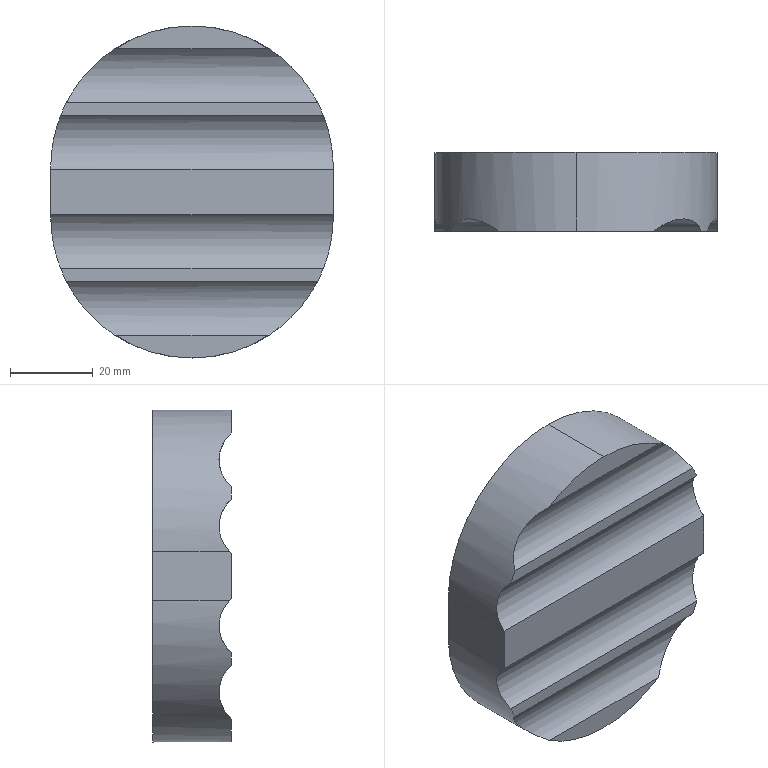Part | SolidWorks | features MirrorStock 1 | 1 solid | 22 faces | box 68 x 19 x 80 mm | volume 59636 mm3 | cylinder 11 | plane 9 | cone 2 | commonest cylinder face diameters 17 x4 68 x3 8.5 x2 62 x2
STEP:
#1=CARTESIAN_POINT('',(0.,7.,-4.25));
#2=VERTEX_POINT('',#1);
#3=CARTESIAN_POINT('',(0.,7.,4.25));
#4=VERTEX_POINT('',#3);
#5=CARTESIAN_POINT('',(0.,7.,0.));
#6=DIRECTION('',(0.,-1.,0.));
#7=DIRECTION('',(0.,0.,-1.));
#8=AXIS2_PLACEMENT_3D('',#5,#6,#7);
#9=CIRCLE('',#8,4.25);
#10=EDGE_CURVE('',#2,#4,#9,.T.);
#11=ORIENTED_EDGE('',*,*,#10,.T.);
#12=CARTESIAN_POINT('',(0.,13.,4.25));
#13=VERTEX_POINT('',#12);
#14=CARTESIAN_POINT('',(0.,13.,4.25));
#15=DIRECTION('',(0.,1.,0.));
#16=VECTOR('',#15,1000.);
#17=LINE('',#14,#16);
#18=EDGE_CURVE('',#4,#13,#17,.T.);
#19=ORIENTED_EDGE('',*,*,#18,.T.);
#20=CARTESIAN_POINT('',(0.,13.,-4.25));
#21=VERTEX_POINT('',#20);
#22=CARTESIAN_POINT('',(0.,13.,0.));
#23=DIRECTION('',(0.,-1.,0.));
#24=DIRECTION('',(0.,0.,-1.));
#25=AXIS2_PLACEMENT_3D('',#22,#23,#24);
#26=CIRCLE('',#25,4.25);
#27=EDGE_CURVE('',#21,#13,#26,.T.);
#28=ORIENTED_EDGE('',*,*,#27,.F.);
#29=CARTESIAN_POINT('',(0.,13.,-4.25));
#30=DIRECTION('',(0.,1.,0.));
#31=VECTOR('',#30,1000.);
#32=LINE('',#29,#31);
#33=EDGE_CURVE('',#2,#21,#32,.T.);
#34=ORIENTED_EDGE('',*,*,#33,.F.);
#35=EDGE_LOOP('',(#11,#19,#28,#34));
#36=FACE_OUTER_BOUND('',#35,.T.);
#37=CARTESIAN_POINT('',(0.,13.,0.));
#38=DIRECTION('',(0.,1.,0.));
#39=DIRECTION('',(0.,0.,-1.));
#40=AXIS2_PLACEMENT_3D('',#37,#38,#39);
#41=CYLINDRICAL_SURFACE('',#40,4.25);
#42=ADVANCED_FACE('',(#36),#41,.F.);
#43=CARTESIAN_POINT('',(0.,4.446,0.));
#44=VERTEX_POINT('',#43);
#45=CARTESIAN_POINT('',(0.,7.,-4.25));
#46=DIRECTION('',(0.,0.515,-0.8572));
#47=VECTOR('',#46,1000.);
#48=LINE('',#45,#47);
#49=EDGE_CURVE('',#44,#2,#48,.T.);
#50=ORIENTED_EDGE('',*,*,#49,.F.);
#51=CARTESIAN_POINT('',(0.,7.,4.25));
#52=DIRECTION('',(0.,0.515,0.8572));
#53=VECTOR('',#52,1000.);
#54=LINE('',#51,#53);
#55=EDGE_CURVE('',#44,#4,#54,.T.);
#56=ORIENTED_EDGE('',*,*,#55,.T.);
#57=ORIENTED_EDGE('',*,*,#10,.F.);
#58=EDGE_LOOP('',(#50,#56,#57));
#59=FACE_OUTER_BOUND('',#58,.T.);
#60=CARTESIAN_POINT('',(0.,7.,0.));
#61=DIRECTION('',(0.,1.,0.));
#62=DIRECTION('',(0.,0.,-1.));
#63=AXIS2_PLACEMENT_3D('',#60,#61,#62);
#64=CONICAL_SURFACE('',#63,4.25,1.03);
#65=ADVANCED_FACE('',(#59),#64,.F.);
#66=CARTESIAN_POINT('',(0.,13.,-31.));
#67=VERTEX_POINT('',#66);
#68=CARTESIAN_POINT('',(0.,13.,31.));
#69=VERTEX_POINT('',#68);
#70=CARTESIAN_POINT('',(0.,13.,0.));
#71=DIRECTION('',(0.,-1.,0.));
#72=DIRECTION('',(0.,0.,-1.));
#73=AXIS2_PLACEMENT_3D('',#70,#71,#72);
#74=CIRCLE('',#73,31.);
#75=EDGE_CURVE('',#67,#69,#74,.T.);
#76=ORIENTED_EDGE('',*,*,#75,.T.);
#77=CARTESIAN_POINT('',(0.,19.,31.));
#78=VERTEX_POINT('',#77);
#79=CARTESIAN_POINT('',(0.,13.,31.));
#80=DIRECTION('',(0.,1.,0.));
#81=VECTOR('',#80,1000.);
#82=LINE('',#79,#81);
#83=EDGE_CURVE('',#69,#78,#82,.T.);
#84=ORIENTED_EDGE('',*,*,#83,.T.);
#85=CARTESIAN_POINT('',(0.,19.,-31.));
#86=VERTEX_POINT('',#85);
#87=CARTESIAN_POINT('',(0.,19.,0.));
#88=DIRECTION('',(0.,-1.,0.));
#89=DIRECTION('',(0.,0.,-1.));
#90=AXIS2_PLACEMENT_3D('',#87,#88,#89);
#91=CIRCLE('',#90,31.);
#92=EDGE_CURVE('',#86,#78,#91,.T.);
#93=ORIENTED_EDGE('',*,*,#92,.F.);
#94=CARTESIAN_POINT('',(0.,13.,-31.));
#95=DIRECTION('',(0.,1.,0.));
#96=VECTOR('',#95,1000.);
#97=LINE('',#94,#96);
#98=EDGE_CURVE('',#67,#86,#97,.T.);
#99=ORIENTED_EDGE('',*,*,#98,.F.);
#100=EDGE_LOOP('',(#76,#84,#93,#99));
#101=FACE_OUTER_BOUND('',#100,.T.);
#102=CARTESIAN_POINT('',(0.,13.,0.));
#103=DIRECTION('',(0.,1.,0.));
#104=DIRECTION('',(0.,0.,-1.));
#105=AXIS2_PLACEMENT_3D('',#102,#103,#104);
#106=CYLINDRICAL_SURFACE('',#105,31.);
#107=ADVANCED_FACE('',(#101),#106,.F.);
#108=CARTESIAN_POINT('',(34.,19.,6.));
#109=VERTEX_POINT('',#108);
#110=CARTESIAN_POINT('',(0.,19.,40.));
#111=VERTEX_POINT('',#110);
#112=CARTESIAN_POINT('',(0.,19.,6.));
#113=DIRECTION('',(0.,-1.,0.));
#114=DIRECTION('',(0.,0.,-1.));
#115=AXIS2_PLACEMENT_3D('',#112,#113,#114);
#116=CIRCLE('',#115,34.);
#117=EDGE_CURVE('',#109,#111,#116,.T.);
#118=ORIENTED_EDGE('',*,*,#117,.T.);
#119=CARTESIAN_POINT('',(0.,0.,40.));
#120=VERTEX_POINT('',#119);
#121=CARTESIAN_POINT('',(0.,19.,40.));
#122=DIRECTION('',(0.,-1.,0.));
#123=VECTOR('',#122,1000.);
#124=LINE('',#121,#123);
#125=EDGE_CURVE('',#111,#120,#124,.T.);
#126=ORIENTED_EDGE('',*,*,#125,.T.);
#127=CARTESIAN_POINT('',(18.57,0.,34.481));
#128=VERTEX_POINT('',#127);
#129=CARTESIAN_POINT('',(0.,0.,6.));
#130=DIRECTION('',(0.,-1.,0.));
#131=DIRECTION('',(0.,0.,-1.));
#132=AXIS2_PLACEMENT_3D('',#129,#130,#131);
#133=CIRCLE('',#132,34.);
#134=EDGE_CURVE('',#128,#120,#133,.T.);
#135=ORIENTED_EDGE('',*,*,#134,.F.);
#136=CARTESIAN_POINT('',(30.251,0.,21.519));
#137=VERTEX_POINT('',#136);
#138=CARTESIAN_POINT('',(18.57,0.,34.481));
#139=CARTESIAN_POINT('',(19.132,0.4318,34.114));
#140=CARTESIAN_POINT('',(19.701,0.8113,33.719));
#141=CARTESIAN_POINT('',(20.842,1.486,32.872));
#142=CARTESIAN_POINT('',(21.414,1.781,32.419));
#143=CARTESIAN_POINT('',(22.557,2.287,31.451));
#144=CARTESIAN_POINT('',(23.13,2.498,30.932));
#145=CARTESIAN_POINT('',(24.241,2.815,29.853));
#146=CARTESIAN_POINT('',(24.783,2.922,29.29));
#147=CARTESIAN_POINT('',(25.572,2.995,28.41));
#148=CARTESIAN_POINT('',(25.832,3.005,28.111));
#149=CARTESIAN_POINT('',(26.343,2.991,27.499));
#150=CARTESIAN_POINT('',(26.593,2.967,27.189));
#151=CARTESIAN_POINT('',(27.319,2.843,26.256));
#152=CARTESIAN_POINT('',(27.773,2.69,25.628));
#153=CARTESIAN_POINT('',(28.41,2.333,24.682));
#154=CARTESIAN_POINT('',(28.615,2.192,24.366));
#155=CARTESIAN_POINT('',(29.,1.871,23.752));
#156=CARTESIAN_POINT('',(29.182,1.689,23.451));
#157=CARTESIAN_POINT('',(29.524,1.283,22.865));
#158=CARTESIAN_POINT('',(29.686,1.057,22.579));
#159=CARTESIAN_POINT('',(29.987,0.5594,22.027));
#160=CARTESIAN_POINT('',(30.125,0.2903,21.766));
#161=CARTESIAN_POINT('',(30.251,0.,21.519));
#162=B_SPLINE_CURVE_WITH_KNOTS('',3,(#138,#139,#140,#141,#142,#143,#144,#145,#146,#147,#148,#149,#150,#151,#152,#153,#154,#155,#156,#157,#158,#159,#160,#161),.UNSPECIFIED.,.F.,.F.,(4,2,2,2,2,2,2,2,2,2,2,4),(0.,0.002359,0.004718,0.007077,0.009436,0.01062,0.0118,0.01415,0.01533,0.01651,0.01769,0.01887),.UNSPECIFIED.);
#163=EDGE_CURVE('',#128,#137,#162,.T.);
#164=ORIENTED_EDGE('',*,*,#163,.T.);
#165=CARTESIAN_POINT('',(31.626,0.,18.481));
#166=VERTEX_POINT('',#165);
#167=CARTESIAN_POINT('',(0.,0.,6.));
#168=DIRECTION('',(0.,-1.,0.));
#169=DIRECTION('',(0.,0.,-1.));
#170=AXIS2_PLACEMENT_3D('',#167,#168,#169);
#171=CIRCLE('',#170,34.);
#172=EDGE_CURVE('',#166,#137,#171,.T.);
#173=ORIENTED_EDGE('',*,*,#172,.F.);
#174=CARTESIAN_POINT('',(34.,0.5208,6.));
#175=VERTEX_POINT('',#174);
#176=CARTESIAN_POINT('',(31.626,0.,18.481));
#177=CARTESIAN_POINT('',(31.775,0.4439,18.104));
#178=CARTESIAN_POINT('',(31.931,0.8401,17.69));
#179=CARTESIAN_POINT('',(32.167,1.368,17.016));
#180=CARTESIAN_POINT('',(32.246,1.533,16.782));
#181=CARTESIAN_POINT('',(32.405,1.841,16.295));
#182=CARTESIAN_POINT('',(32.484,1.983,16.042));
#183=CARTESIAN_POINT('',(32.717,2.367,15.269));
#184=CARTESIAN_POINT('',(32.865,2.57,14.732));
#185=CARTESIAN_POINT('',(33.072,2.791,13.894));
#186=CARTESIAN_POINT('',(33.139,2.852,13.608));
#187=CARTESIAN_POINT('',(33.267,2.943,13.029));
#188=CARTESIAN_POINT('',(33.327,2.973,12.739));
#189=CARTESIAN_POINT('',(33.495,3.019,11.868));
#190=CARTESIAN_POINT('',(33.592,2.991,11.284));
#191=CARTESIAN_POINT('',(33.715,2.854,10.405));
#192=CARTESIAN_POINT('',(33.752,2.793,10.113));
#193=CARTESIAN_POINT('',(33.816,2.642,9.541));
#194=CARTESIAN_POINT('',(33.844,2.552,9.26));
#195=CARTESIAN_POINT('',(33.893,2.342,8.708));
#196=CARTESIAN_POINT('',(33.914,2.223,8.437));
#197=CARTESIAN_POINT('',(33.948,1.954,7.905));
#198=CARTESIAN_POINT('',(33.961,1.805,7.643));
#199=CARTESIAN_POINT('',(33.992,1.319,6.89));
#200=CARTESIAN_POINT('',(34.,0.9452,6.426));
#201=CARTESIAN_POINT('',(34.,0.5208,6.));
#202=B_SPLINE_CURVE_WITH_KNOTS('',3,(#176,#177,#178,#179,#180,#181,#182,#183,#184,#185,#186,#187,#188,#189,#190,#191,#192,#193,#194,#195,#196,#197,#198,#199,#200,#201),.UNSPECIFIED.,.F.,.F.,(4,2,2,2,2,2,2,2,2,2,2,2,4),(0.,0.001777,0.002665,0.003554,0.005331,0.006219,0.007107,0.008884,0.009773,0.01066,0.01155,0.01244,0.01421),.UNSPECIFIED.);
#203=EDGE_CURVE('',#166,#175,#202,.T.);
#204=ORIENTED_EDGE('',*,*,#203,.T.);
#205=CARTESIAN_POINT('',(34.,19.,6.));
#206=DIRECTION('',(0.,-1.,0.));
#207=VECTOR('',#206,1000.);
#208=LINE('',#205,#207);
#209=EDGE_CURVE('',#109,#175,#208,.T.);
#210=ORIENTED_EDGE('',*,*,#209,.F.);
#211=EDGE_LOOP('',(#118,#126,#135,#164,#173,#204,#210));
#212=FACE_OUTER_BOUND('',#211,.T.);
#213=CARTESIAN_POINT('',(0.,19.,6.));
#214=DIRECTION('',(0.,-1.,0.));
#215=DIRECTION('',(0.,0.,1.));
#216=AXIS2_PLACEMENT_3D('',#213,#214,#215);
#217=CYLINDRICAL_SURFACE('',#216,34.);
#218=ADVANCED_FACE('',(#212),#217,.T.);
#219=ORIENTED_EDGE('',*,*,#125,.F.);
#220=CARTESIAN_POINT('',(-34.,19.,6.));
#221=VERTEX_POINT('',#220);
#222=CARTESIAN_POINT('',(0.,19.,6.));
#223=DIRECTION('',(0.,-1.,0.));
#224=DIRECTION('',(0.,0.,-1.));
#225=AXIS2_PLACEMENT_3D('',#222,#223,#224);
#226=CIRCLE('',#225,34.);
#227=EDGE_CURVE('',#111,#221,#226,.T.);
#228=ORIENTED_EDGE('',*,*,#227,.T.);
#229=CARTESIAN_POINT('',(-34.,0.5208,6.));
#230=VERTEX_POINT('',#229);
#231=CARTESIAN_POINT('',(-34.,19.,6.));
#232=DIRECTION('',(0.,-1.,0.));
#233=VECTOR('',#232,1000.);
#234=LINE('',#231,#233);
#235=EDGE_CURVE('',#221,#230,#234,.T.);
#236=ORIENTED_EDGE('',*,*,#235,.T.);
#237=CARTESIAN_POINT('',(-31.626,0.,18.481));
#238=VERTEX_POINT('',#237);
#239=CARTESIAN_POINT('',(-34.,0.5208,6.));
#240=CARTESIAN_POINT('',(-34.,0.9451,6.426));
#241=CARTESIAN_POINT('',(-33.992,1.317,6.888));
#242=CARTESIAN_POINT('',(-33.962,1.8,7.635));
#243=CARTESIAN_POINT('',(-33.948,1.948,7.893));
#244=CARTESIAN_POINT('',(-33.914,2.218,8.427));
#245=CARTESIAN_POINT('',(-33.894,2.339,8.701));
#246=CARTESIAN_POINT('',(-33.821,2.655,9.532));
#247=CARTESIAN_POINT('',(-33.757,2.806,10.101));
#248=CARTESIAN_POINT('',(-33.635,2.944,10.979));
#249=CARTESIAN_POINT('',(-33.59,2.974,11.276));
#250=CARTESIAN_POINT('',(-33.492,3.004,11.862));
#251=CARTESIAN_POINT('',(-33.44,3.004,12.154));
#252=CARTESIAN_POINT('',(-33.327,2.973,12.736));
#253=CARTESIAN_POINT('',(-33.268,2.943,13.025));
#254=CARTESIAN_POINT('',(-33.141,2.853,13.601));
#255=CARTESIAN_POINT('',(-33.073,2.792,13.889));
#256=CARTESIAN_POINT('',(-32.865,2.57,14.73));
#257=CARTESIAN_POINT('',(-32.717,2.368,15.268));
#258=CARTESIAN_POINT('',(-32.485,1.984,16.04));
#259=CARTESIAN_POINT('',(-32.405,1.842,16.293));
#260=CARTESIAN_POINT('',(-32.247,1.534,16.781));
#261=CARTESIAN_POINT('',(-32.167,1.369,17.015));
#262=CARTESIAN_POINT('',(-31.931,0.8402,17.69));
#263=CARTESIAN_POINT('',(-31.775,0.4438,18.104));
#264=CARTESIAN_POINT('',(-31.626,0.,18.481));
#265=B_SPLINE_CURVE_WITH_KNOTS('',3,(#239,#240,#241,#242,#243,#244,#245,#246,#247,#248,#249,#250,#251,#252,#253,#254,#255,#256,#257,#258,#259,#260,#261,#262,#263,#264),.UNSPECIFIED.,.F.,.F.,(4,2,2,2,2,2,2,2,2,2,2,2,4),(0.,0.001778,0.002667,0.003556,0.005334,0.006222,0.007111,0.008,0.008889,0.01067,0.01156,0.01244,0.01422),.UNSPECIFIED.);
#266=EDGE_CURVE('',#230,#238,#265,.T.);
#267=ORIENTED_EDGE('',*,*,#266,.T.);
#268=CARTESIAN_POINT('',(-30.251,0.,21.519));
#269=VERTEX_POINT('',#268);
#270=CARTESIAN_POINT('',(0.,0.,6.));
#271=DIRECTION('',(0.,-1.,0.));
#272=DIRECTION('',(0.,0.,-1.));
#273=AXIS2_PLACEMENT_3D('',#270,#271,#272);
#274=CIRCLE('',#273,34.);
#275=EDGE_CURVE('',#269,#238,#274,.T.);
#276=ORIENTED_EDGE('',*,*,#275,.F.);
#277=CARTESIAN_POINT('',(-18.57,0.,34.481));
#278=VERTEX_POINT('',#277);
#279=CARTESIAN_POINT('',(-30.251,0.,21.519));
#280=CARTESIAN_POINT('',(-29.999,0.5804,22.012));
#281=CARTESIAN_POINT('',(-29.703,1.069,22.558));
#282=CARTESIAN_POINT('',(-29.189,1.681,23.438));
#283=CARTESIAN_POINT('',(-29.005,1.866,23.744));
#284=CARTESIAN_POINT('',(-28.619,2.189,24.361));
#285=CARTESIAN_POINT('',(-28.417,2.328,24.672));
#286=CARTESIAN_POINT('',(-27.995,2.566,25.298));
#287=CARTESIAN_POINT('',(-27.775,2.665,25.614));
#288=CARTESIAN_POINT('',(-27.317,2.824,26.247));
#289=CARTESIAN_POINT('',(-27.08,2.884,26.563));
#290=CARTESIAN_POINT('',(-26.355,3.008,27.495));
#291=CARTESIAN_POINT('',(-25.85,3.02,28.1));
#292=CARTESIAN_POINT('',(-25.059,2.948,28.982));
#293=CARTESIAN_POINT('',(-24.789,2.909,29.273));
#294=CARTESIAN_POINT('',(-24.243,2.803,29.842));
#295=CARTESIAN_POINT('',(-23.967,2.736,30.119));
#296=CARTESIAN_POINT('',(-23.136,2.5,30.927));
#297=CARTESIAN_POINT('',(-22.573,2.293,31.436));
#298=CARTESIAN_POINT('',(-21.72,1.917,32.161));
#299=CARTESIAN_POINT('',(-21.433,1.78,32.396));
#300=CARTESIAN_POINT('',(-20.858,1.484,32.853));
#301=CARTESIAN_POINT('',(-20.568,1.324,33.075));
#302=CARTESIAN_POINT('',(-19.703,0.8129,33.718));
#303=CARTESIAN_POINT('',(-19.131,0.4312,34.115));
#304=CARTESIAN_POINT('',(-18.57,0.,34.481));
#305=B_SPLINE_CURVE_WITH_KNOTS('',3,(#279,#280,#281,#282,#283,#284,#285,#286,#287,#288,#289,#290,#291,#292,#293,#294,#295,#296,#297,#298,#299,#300,#301,#302,#303,#304),.UNSPECIFIED.,.F.,.F.,(4,2,2,2,2,2,2,2,2,2,2,2,4),(0.,0.002368,0.003552,0.004736,0.005921,0.007105,0.009473,0.01066,0.01184,0.01421,0.01539,0.01658,0.01895),.UNSPECIFIED.);
#306=EDGE_CURVE('',#269,#278,#305,.T.);
#307=ORIENTED_EDGE('',*,*,#306,.T.);
#308=CARTESIAN_POINT('',(0.,0.,6.));
#309=DIRECTION('',(0.,-1.,0.));
#310=DIRECTION('',(0.,0.,-1.));
#311=AXIS2_PLACEMENT_3D('',#308,#309,#310);
#312=CIRCLE('',#311,34.);
#313=EDGE_CURVE('',#120,#278,#312,.T.);
#314=ORIENTED_EDGE('',*,*,#313,.F.);
#315=EDGE_LOOP('',(#219,#228,#236,#267,#276,#307,#314));
#316=FACE_OUTER_BOUND('',#315,.T.);
#317=CARTESIAN_POINT('',(0.,19.,6.));
#318=DIRECTION('',(0.,-1.,0.));
#319=DIRECTION('',(0.,0.,1.));
#320=AXIS2_PLACEMENT_3D('',#317,#318,#319);
#321=CYLINDRICAL_SURFACE('',#320,34.);
#322=ADVANCED_FACE('',(#316),#321,.T.);
#323=CARTESIAN_POINT('',(34.,0.,5.519));
#324=VERTEX_POINT('',#323);
#325=CARTESIAN_POINT('',(-34.,0.,5.519));
#326=VERTEX_POINT('',#325);
#327=CARTESIAN_POINT('',(-34.,0.,5.519));
#328=DIRECTION('',(-1.,0.,0.));
#329=VECTOR('',#328,1000.);
#330=LINE('',#327,#329);
#331=EDGE_CURVE('',#324,#326,#330,.T.);
#332=ORIENTED_EDGE('',*,*,#331,.T.);
#333=CARTESIAN_POINT('',(-34.,0.,-5.519));
#334=VERTEX_POINT('',#333);
#335=CARTESIAN_POINT('',(-34.,0.,-6.));
#336=DIRECTION('',(0.,0.,-1.));
#337=VECTOR('',#336,1000.);
#338=LINE('',#335,#337);
#339=EDGE_CURVE('',#326,#334,#338,.T.);
#340=ORIENTED_EDGE('',*,*,#339,.T.);
#341=CARTESIAN_POINT('',(34.,0.,-5.519));
#342=VERTEX_POINT('',#341);
#343=CARTESIAN_POINT('',(-34.,0.,-5.519));
#344=DIRECTION('',(-1.,0.,0.));
#345=VECTOR('',#344,1000.);
#346=LINE('',#343,#345);
#347=EDGE_CURVE('',#342,#334,#346,.T.);
#348=ORIENTED_EDGE('',*,*,#347,.F.);
#349=CARTESIAN_POINT('',(34.,0.,-6.));
#350=DIRECTION('',(0.,0.,1.));
#351=VECTOR('',#350,1000.);
#352=LINE('',#349,#351);
#353=EDGE_CURVE('',#342,#324,#352,.T.);
#354=ORIENTED_EDGE('',*,*,#353,.T.);
#355=EDGE_LOOP('',(#332,#340,#348,#354));
#356=FACE_OUTER_BOUND('',#355,.T.);
#357=CARTESIAN_POINT('',(0.,0.,6.));
#358=DIRECTION('',(0.,1.,0.));
#359=DIRECTION('',(0.,0.,-1.));
#360=AXIS2_PLACEMENT_3D('',#357,#358,#359);
#361=PLANE('',#360);
#362=ADVANCED_FACE('',(#356),#361,.F.);
#363=CARTESIAN_POINT('',(-34.,0.,18.481));
#364=DIRECTION('',(1.,0.,0.));
#365=VECTOR('',#364,1000.);
#366=LINE('',#363,#365);
#367=EDGE_CURVE('',#238,#166,#366,.T.);
#368=ORIENTED_EDGE('',*,*,#367,.T.);
#369=ORIENTED_EDGE('',*,*,#172,.T.);
#370=CARTESIAN_POINT('',(-34.,0.,21.519));
#371=DIRECTION('',(-1.,0.,0.));
#372=VECTOR('',#371,1000.);
#373=LINE('',#370,#372);
#374=EDGE_CURVE('',#137,#269,#373,.T.);
#375=ORIENTED_EDGE('',*,*,#374,.T.);
#376=ORIENTED_EDGE('',*,*,#275,.T.);
#377=EDGE_LOOP('',(#368,#369,#375,#376));
#378=FACE_OUTER_BOUND('',#377,.T.);
#379=CARTESIAN_POINT('',(0.,0.,6.));
#380=DIRECTION('',(0.,1.,0.));
#381=DIRECTION('',(0.,0.,-1.));
#382=AXIS2_PLACEMENT_3D('',#379,#380,#381);
#383=PLANE('',#382);
#384=ADVANCED_FACE('',(#378),#383,.F.);
#385=CARTESIAN_POINT('',(-31.626,0.,-18.481));
#386=VERTEX_POINT('',#385);
#387=CARTESIAN_POINT('',(-30.251,0.,-21.519));
#388=VERTEX_POINT('',#387);
#389=CARTESIAN_POINT('',(0.,0.,-6.));
#390=DIRECTION('',(0.,-1.,0.));
#391=DIRECTION('',(0.,0.,1.));
#392=AXIS2_PLACEMENT_3D('',#389,#390,#391);
#393=CIRCLE('',#392,34.);
#394=EDGE_CURVE('',#386,#388,#393,.T.);
#395=ORIENTED_EDGE('',*,*,#394,.T.);
#396=CARTESIAN_POINT('',(30.251,0.,-21.519));
#397=VERTEX_POINT('',#396);
#398=CARTESIAN_POINT('',(-34.,0.,-21.519));
#399=DIRECTION('',(-1.,0.,0.));
#400=VECTOR('',#399,1000.);
#401=LINE('',#398,#400);
#402=EDGE_CURVE('',#397,#388,#401,.T.);
#403=ORIENTED_EDGE('',*,*,#402,.F.);
#404=CARTESIAN_POINT('',(31.626,0.,-18.481));
#405=VERTEX_POINT('',#404);
#406=CARTESIAN_POINT('',(0.,0.,-6.));
#407=DIRECTION('',(0.,-1.,0.));
#408=DIRECTION('',(0.,0.,1.));
#409=AXIS2_PLACEMENT_3D('',#406,#407,#408);
#410=CIRCLE('',#409,34.);
#411=EDGE_CURVE('',#397,#405,#410,.T.);
#412=ORIENTED_EDGE('',*,*,#411,.T.);
#413=CARTESIAN_POINT('',(-34.,0.,-18.481));
#414=DIRECTION('',(1.,0.,0.));
#415=VECTOR('',#414,1000.);
#416=LINE('',#413,#415);
#417=EDGE_CURVE('',#386,#405,#416,.T.);
#418=ORIENTED_EDGE('',*,*,#417,.F.);
#419=EDGE_LOOP('',(#395,#403,#412,#418));
#420=FACE_OUTER_BOUND('',#419,.T.);
#421=CARTESIAN_POINT('',(0.,0.,6.));
#422=DIRECTION('',(0.,1.,0.));
#423=DIRECTION('',(0.,0.,-1.));
#424=AXIS2_PLACEMENT_3D('',#421,#422,#423);
#425=PLANE('',#424);
#426=ADVANCED_FACE('',(#420),#425,.F.);
#427=CARTESIAN_POINT('',(-34.,-5.5,12.));
#428=DIRECTION('',(1.,0.,0.));
#429=DIRECTION('',(0.,0.,1.));
#430=AXIS2_PLACEMENT_3D('',#427,#428,#429);
#431=CIRCLE('',#430,8.5);
#432=EDGE_CURVE('',#326,#230,#431,.T.);
#433=ORIENTED_EDGE('',*,*,#432,.T.);
#434=ORIENTED_EDGE('',*,*,#235,.F.);
#435=CARTESIAN_POINT('',(-34.,19.,-6.));
#436=VERTEX_POINT('',#435);
#437=CARTESIAN_POINT('',(-34.,19.,-6.));
#438=DIRECTION('',(0.,0.,-1.));
#439=VECTOR('',#438,1000.);
#440=LINE('',#437,#439);
#441=EDGE_CURVE('',#221,#436,#440,.T.);
#442=ORIENTED_EDGE('',*,*,#441,.T.);
#443=CARTESIAN_POINT('',(-34.,0.5208,-6.));
#444=VERTEX_POINT('',#443);
#445=CARTESIAN_POINT('',(-34.,19.,-6.));
#446=DIRECTION('',(0.,-1.,0.));
#447=VECTOR('',#446,1000.);
#448=LINE('',#445,#447);
#449=EDGE_CURVE('',#436,#444,#448,.T.);
#450=ORIENTED_EDGE('',*,*,#449,.T.);
#451=CARTESIAN_POINT('',(-34.,-5.5,-12.));
#452=DIRECTION('',(-1.,0.,0.));
#453=DIRECTION('',(0.,0.,1.));
#454=AXIS2_PLACEMENT_3D('',#451,#452,#453);
#455=CIRCLE('',#454,8.5);
#456=EDGE_CURVE('',#334,#444,#455,.T.);
#457=ORIENTED_EDGE('',*,*,#456,.F.);
#458=ORIENTED_EDGE('',*,*,#339,.F.);
#459=EDGE_LOOP('',(#433,#434,#442,#450,#457,#458));
#460=FACE_OUTER_BOUND('',#459,.T.);
#461=CARTESIAN_POINT('',(-34.,19.,-6.));
#462=DIRECTION('',(1.,0.,0.));
#463=DIRECTION('',(0.,0.,1.));
#464=AXIS2_PLACEMENT_3D('',#461,#462,#463);
#465=PLANE('',#464);
#466=ADVANCED_FACE('',(#460),#465,.F.);
#467=CARTESIAN_POINT('',(34.,-5.5,12.));
#468=DIRECTION('',(-1.,0.,0.));
#469=DIRECTION('',(0.,0.,-1.));
#470=AXIS2_PLACEMENT_3D('',#467,#468,#469);
#471=CIRCLE('',#470,8.5);
#472=EDGE_CURVE('',#175,#324,#471,.T.);
#473=ORIENTED_EDGE('',*,*,#472,.T.);
#474=ORIENTED_EDGE('',*,*,#353,.F.);
#475=CARTESIAN_POINT('',(34.,0.5208,-6.));
#476=VERTEX_POINT('',#475);
#477=CARTESIAN_POINT('',(34.,-5.5,-12.));
#478=DIRECTION('',(1.,0.,0.));
#479=DIRECTION('',(0.,0.,-1.));
#480=AXIS2_PLACEMENT_3D('',#477,#478,#479);
#481=CIRCLE('',#480,8.5);
#482=EDGE_CURVE('',#476,#342,#481,.T.);
#483=ORIENTED_EDGE('',*,*,#482,.F.);
#484=CARTESIAN_POINT('',(34.,19.,-6.));
#485=VERTEX_POINT('',#484);
#486=CARTESIAN_POINT('',(34.,19.,-6.));
#487=DIRECTION('',(0.,-1.,0.));
#488=VECTOR('',#487,1000.);
#489=LINE('',#486,#488);
#490=EDGE_CURVE('',#485,#476,#489,.T.);
#491=ORIENTED_EDGE('',*,*,#490,.F.);
#492=CARTESIAN_POINT('',(34.,19.,-6.));
#493=DIRECTION('',(0.,0.,1.));
#494=VECTOR('',#493,1000.);
#495=LINE('',#492,#494);
#496=EDGE_CURVE('',#485,#109,#495,.T.);
#497=ORIENTED_EDGE('',*,*,#496,.T.);
#498=ORIENTED_EDGE('',*,*,#209,.T.);
#499=EDGE_LOOP('',(#473,#474,#483,#491,#497,#498));
#500=FACE_OUTER_BOUND('',#499,.T.);
#501=CARTESIAN_POINT('',(34.,19.,-6.));
#502=DIRECTION('',(-1.,0.,0.));
#503=DIRECTION('',(0.,0.,-1.));
#504=AXIS2_PLACEMENT_3D('',#501,#502,#503);
#505=PLANE('',#504);
#506=ADVANCED_FACE('',(#500),#505,.F.);
#507=CARTESIAN_POINT('',(-34.,0.,34.481));
#508=DIRECTION('',(1.,0.,0.));
#509=VECTOR('',#508,1000.);
#510=LINE('',#507,#509);
#511=EDGE_CURVE('',#278,#128,#510,.T.);
#512=ORIENTED_EDGE('',*,*,#511,.T.);
#513=ORIENTED_EDGE('',*,*,#134,.T.);
#514=ORIENTED_EDGE('',*,*,#313,.T.);
#515=EDGE_LOOP('',(#512,#513,#514));
#516=FACE_OUTER_BOUND('',#515,.T.);
#517=CARTESIAN_POINT('',(0.,0.,6.));
#518=DIRECTION('',(0.,1.,0.));
#519=DIRECTION('',(0.,0.,-1.));
#520=AXIS2_PLACEMENT_3D('',#517,#518,#519);
#521=PLANE('',#520);
#522=ADVANCED_FACE('',(#516),#521,.F.);
#523=CARTESIAN_POINT('',(-18.57,0.,-34.481));
#524=VERTEX_POINT('',#523);
#525=CARTESIAN_POINT('',(18.57,0.,-34.481));
#526=VERTEX_POINT('',#525);
#527=CARTESIAN_POINT('',(0.,0.,-6.));
#528=DIRECTION('',(0.,-1.,0.));
#529=DIRECTION('',(0.,0.,1.));
#530=AXIS2_PLACEMENT_3D('',#527,#528,#529);
#531=CIRCLE('',#530,34.);
#532=EDGE_CURVE('',#524,#526,#531,.T.);
#533=ORIENTED_EDGE('',*,*,#532,.T.);
#534=CARTESIAN_POINT('',(-34.,0.,-34.481));
#535=DIRECTION('',(1.,0.,0.));
#536=VECTOR('',#535,1000.);
#537=LINE('',#534,#536);
#538=EDGE_CURVE('',#524,#526,#537,.T.);
#539=ORIENTED_EDGE('',*,*,#538,.F.);
#540=EDGE_LOOP('',(#533,#539));
#541=FACE_OUTER_BOUND('',#540,.T.);
#542=CARTESIAN_POINT('',(0.,0.,6.));
#543=DIRECTION('',(0.,1.,0.));
#544=DIRECTION('',(0.,0.,-1.));
#545=AXIS2_PLACEMENT_3D('',#542,#543,#544);
#546=PLANE('',#545);
#547=ADVANCED_FACE('',(#541),#546,.F.);
#548=ORIENTED_EDGE('',*,*,#449,.F.);
#549=CARTESIAN_POINT('',(0.,19.,-6.));
#550=DIRECTION('',(0.,-1.,0.));
#551=DIRECTION('',(0.,0.,1.));
#552=AXIS2_PLACEMENT_3D('',#549,#550,#551);
#553=CIRCLE('',#552,34.);
#554=EDGE_CURVE('',#436,#485,#553,.T.);
#555=ORIENTED_EDGE('',*,*,#554,.T.);
#556=ORIENTED_EDGE('',*,*,#490,.T.);
#557=CARTESIAN_POINT('',(31.626,0.,-18.481));
#558=CARTESIAN_POINT('',(31.775,0.4439,-18.104));
#559=CARTESIAN_POINT('',(31.931,0.8401,-17.69));
#560=CARTESIAN_POINT('',(32.167,1.368,-17.016));
#561=CARTESIAN_POINT('',(32.246,1.533,-16.782));
#562=CARTESIAN_POINT('',(32.405,1.841,-16.295));
#563=CARTESIAN_POINT('',(32.484,1.983,-16.042));
#564=CARTESIAN_POINT('',(32.717,2.367,-15.269));
#565=CARTESIAN_POINT('',(32.865,2.57,-14.732));
#566=CARTESIAN_POINT('',(33.072,2.791,-13.894));
#567=CARTESIAN_POINT('',(33.139,2.852,-13.608));
#568=CARTESIAN_POINT('',(33.267,2.943,-13.029));
#569=CARTESIAN_POINT('',(33.327,2.973,-12.739));
#570=CARTESIAN_POINT('',(33.495,3.019,-11.868));
#571=CARTESIAN_POINT('',(33.592,2.991,-11.284));
#572=CARTESIAN_POINT('',(33.715,2.854,-10.405));
#573=CARTESIAN_POINT('',(33.752,2.793,-10.113));
#574=CARTESIAN_POINT('',(33.816,2.642,-9.541));
#575=CARTESIAN_POINT('',(33.844,2.552,-9.26));
#576=CARTESIAN_POINT('',(33.893,2.342,-8.708));
#577=CARTESIAN_POINT('',(33.914,2.223,-8.437));
#578=CARTESIAN_POINT('',(33.948,1.954,-7.905));
#579=CARTESIAN_POINT('',(33.961,1.805,-7.643));
#580=CARTESIAN_POINT('',(33.992,1.319,-6.89));
#581=CARTESIAN_POINT('',(34.,0.9452,-6.426));
#582=CARTESIAN_POINT('',(34.,0.5208,-6.));
#583=B_SPLINE_CURVE_WITH_KNOTS('',3,(#557,#558,#559,#560,#561,#562,#563,#564,#565,#566,#567,#568,#569,#570,#571,#572,#573,#574,#575,#576,#577,#578,#579,#580,#581,#582),.UNSPECIFIED.,.F.,.F.,(4,2,2,2,2,2,2,2,2,2,2,2,4),(0.,0.001777,0.002665,0.003554,0.005331,0.006219,0.007107,0.008884,0.009773,0.01066,0.01155,0.01244,0.01421),.UNSPECIFIED.);
#584=EDGE_CURVE('',#405,#476,#583,.T.);
#585=ORIENTED_EDGE('',*,*,#584,.F.);
#586=ORIENTED_EDGE('',*,*,#411,.F.);
#587=CARTESIAN_POINT('',(18.57,0.,-34.481));
#588=CARTESIAN_POINT('',(19.132,0.4318,-34.114));
#589=CARTESIAN_POINT('',(19.701,0.8113,-33.719));
#590=CARTESIAN_POINT('',(20.842,1.486,-32.872));
#591=CARTESIAN_POINT('',(21.414,1.781,-32.419));
#592=CARTESIAN_POINT('',(22.557,2.287,-31.451));
#593=CARTESIAN_POINT('',(23.13,2.498,-30.932));
#594=CARTESIAN_POINT('',(24.241,2.815,-29.853));
#595=CARTESIAN_POINT('',(24.783,2.922,-29.29));
#596=CARTESIAN_POINT('',(25.572,2.995,-28.41));
#597=CARTESIAN_POINT('',(25.832,3.005,-28.111));
#598=CARTESIAN_POINT('',(26.343,2.991,-27.499));
#599=CARTESIAN_POINT('',(26.593,2.967,-27.189));
#600=CARTESIAN_POINT('',(27.319,2.843,-26.256));
#601=CARTESIAN_POINT('',(27.773,2.69,-25.628));
#602=CARTESIAN_POINT('',(28.41,2.333,-24.682));
#603=CARTESIAN_POINT('',(28.615,2.192,-24.366));
#604=CARTESIAN_POINT('',(29.,1.871,-23.752));
#605=CARTESIAN_POINT('',(29.182,1.689,-23.451));
#606=CARTESIAN_POINT('',(29.524,1.283,-22.865));
#607=CARTESIAN_POINT('',(29.686,1.057,-22.579));
#608=CARTESIAN_POINT('',(29.987,0.5594,-22.027));
#609=CARTESIAN_POINT('',(30.125,0.2903,-21.766));
#610=CARTESIAN_POINT('',(30.251,0.,-21.519));
#611=B_SPLINE_CURVE_WITH_KNOTS('',3,(#587,#588,#589,#590,#591,#592,#593,#594,#595,#596,#597,#598,#599,#600,#601,#602,#603,#604,#605,#606,#607,#608,#609,#610),.UNSPECIFIED.,.F.,.F.,(4,2,2,2,2,2,2,2,2,2,2,4),(0.,0.002359,0.004718,0.007077,0.009436,0.01062,0.0118,0.01415,0.01533,0.01651,0.01769,0.01887),.UNSPECIFIED.);
#612=EDGE_CURVE('',#526,#397,#611,.T.);
#613=ORIENTED_EDGE('',*,*,#612,.F.);
#614=ORIENTED_EDGE('',*,*,#532,.F.);
#615=CARTESIAN_POINT('',(-30.251,0.,-21.519));
#616=CARTESIAN_POINT('',(-29.999,0.5804,-22.012));
#617=CARTESIAN_POINT('',(-29.703,1.069,-22.558));
#618=CARTESIAN_POINT('',(-29.189,1.681,-23.438));
#619=CARTESIAN_POINT('',(-29.005,1.866,-23.744));
#620=CARTESIAN_POINT('',(-28.619,2.189,-24.361));
#621=CARTESIAN_POINT('',(-28.417,2.328,-24.672));
#622=CARTESIAN_POINT('',(-27.995,2.566,-25.298));
#623=CARTESIAN_POINT('',(-27.775,2.665,-25.614));
#624=CARTESIAN_POINT('',(-27.317,2.824,-26.247));
#625=CARTESIAN_POINT('',(-27.08,2.884,-26.563));
#626=CARTESIAN_POINT('',(-26.355,3.008,-27.495));
#627=CARTESIAN_POINT('',(-25.85,3.02,-28.1));
#628=CARTESIAN_POINT('',(-25.059,2.948,-28.982));
#629=CARTESIAN_POINT('',(-24.789,2.909,-29.273));
#630=CARTESIAN_POINT('',(-24.243,2.803,-29.842));
#631=CARTESIAN_POINT('',(-23.967,2.736,-30.119));
#632=CARTESIAN_POINT('',(-23.136,2.5,-30.927));
#633=CARTESIAN_POINT('',(-22.573,2.293,-31.436));
#634=CARTESIAN_POINT('',(-21.72,1.917,-32.161));
#635=CARTESIAN_POINT('',(-21.433,1.78,-32.396));
#636=CARTESIAN_POINT('',(-20.858,1.484,-32.853));
#637=CARTESIAN_POINT('',(-20.568,1.324,-33.075));
#638=CARTESIAN_POINT('',(-19.703,0.8129,-33.718));
#639=CARTESIAN_POINT('',(-19.131,0.4312,-34.115));
#640=CARTESIAN_POINT('',(-18.57,0.,-34.481));
#641=B_SPLINE_CURVE_WITH_KNOTS('',3,(#615,#616,#617,#618,#619,#620,#621,#622,#623,#624,#625,#626,#627,#628,#629,#630,#631,#632,#633,#634,#635,#636,#637,#638,#639,#640),.UNSPECIFIED.,.F.,.F.,(4,2,2,2,2,2,2,2,2,2,2,2,4),(0.,0.002368,0.003552,0.004736,0.005921,0.007105,0.009473,0.01066,0.01184,0.01421,0.01539,0.01658,0.01895),.UNSPECIFIED.);
#642=EDGE_CURVE('',#388,#524,#641,.T.);
#643=ORIENTED_EDGE('',*,*,#642,.F.);
#644=ORIENTED_EDGE('',*,*,#394,.F.);
#645=CARTESIAN_POINT('',(-34.,0.5208,-6.));
#646=CARTESIAN_POINT('',(-34.,0.9451,-6.426));
#647=CARTESIAN_POINT('',(-33.992,1.317,-6.888));
#648=CARTESIAN_POINT('',(-33.962,1.8,-7.635));
#649=CARTESIAN_POINT('',(-33.948,1.948,-7.893));
#650=CARTESIAN_POINT('',(-33.914,2.218,-8.427));
#651=CARTESIAN_POINT('',(-33.894,2.339,-8.701));
#652=CARTESIAN_POINT('',(-33.821,2.655,-9.532));
#653=CARTESIAN_POINT('',(-33.757,2.806,-10.101));
#654=CARTESIAN_POINT('',(-33.635,2.944,-10.979));
#655=CARTESIAN_POINT('',(-33.59,2.974,-11.276));
#656=CARTESIAN_POINT('',(-33.492,3.004,-11.862));
#657=CARTESIAN_POINT('',(-33.44,3.004,-12.154));
#658=CARTESIAN_POINT('',(-33.327,2.973,-12.736));
#659=CARTESIAN_POINT('',(-33.268,2.943,-13.025));
#660=CARTESIAN_POINT('',(-33.141,2.853,-13.601));
#661=CARTESIAN_POINT('',(-33.073,2.792,-13.889));
#662=CARTESIAN_POINT('',(-32.865,2.57,-14.73));
#663=CARTESIAN_POINT('',(-32.717,2.368,-15.268));
#664=CARTESIAN_POINT('',(-32.485,1.984,-16.04));
#665=CARTESIAN_POINT('',(-32.405,1.842,-16.293));
#666=CARTESIAN_POINT('',(-32.247,1.534,-16.781));
#667=CARTESIAN_POINT('',(-32.167,1.369,-17.015));
#668=CARTESIAN_POINT('',(-31.931,0.8402,-17.69));
#669=CARTESIAN_POINT('',(-31.775,0.4438,-18.104));
#670=CARTESIAN_POINT('',(-31.626,0.,-18.481));
#671=B_SPLINE_CURVE_WITH_KNOTS('',3,(#645,#646,#647,#648,#649,#650,#651,#652,#653,#654,#655,#656,#657,#658,#659,#660,#661,#662,#663,#664,#665,#666,#667,#668,#669,#670),.UNSPECIFIED.,.F.,.F.,(4,2,2,2,2,2,2,2,2,2,2,2,4),(0.,0.001778,0.002667,0.003556,0.005334,0.006222,0.007111,0.008,0.008889,0.01067,0.01156,0.01244,0.01422),.UNSPECIFIED.);
#672=EDGE_CURVE('',#444,#386,#671,.T.);
#673=ORIENTED_EDGE('',*,*,#672,.F.);
#674=EDGE_LOOP('',(#548,#555,#556,#585,#586,#613,#614,#643,#644,#673));
#675=FACE_OUTER_BOUND('',#674,.T.);
#676=CARTESIAN_POINT('',(0.,19.,-6.));
#677=DIRECTION('',(0.,-1.,0.));
#678=DIRECTION('',(0.,0.,1.));
#679=AXIS2_PLACEMENT_3D('',#676,#677,#678);
#680=CYLINDRICAL_SURFACE('',#679,34.);
#681=ADVANCED_FACE('',(#675),#680,.T.);
#682=ORIENTED_EDGE('',*,*,#92,.T.);
#683=CARTESIAN_POINT('',(0.,19.,0.));
#684=DIRECTION('',(0.,-1.,0.));
#685=DIRECTION('',(0.,0.,-1.));
#686=AXIS2_PLACEMENT_3D('',#683,#684,#685);
#687=CIRCLE('',#686,31.);
#688=EDGE_CURVE('',#78,#86,#687,.T.);
#689=ORIENTED_EDGE('',*,*,#688,.T.);
#690=EDGE_LOOP('',(#682,#689));
#691=FACE_BOUND('',#690,.T.);
#692=ORIENTED_EDGE('',*,*,#117,.F.);
#693=ORIENTED_EDGE('',*,*,#496,.F.);
#694=ORIENTED_EDGE('',*,*,#554,.F.);
#695=ORIENTED_EDGE('',*,*,#441,.F.);
#696=ORIENTED_EDGE('',*,*,#227,.F.);
#697=EDGE_LOOP('',(#692,#693,#694,#695,#696));
#698=FACE_OUTER_BOUND('',#697,.T.);
#699=CARTESIAN_POINT('',(0.,19.,6.));
#700=DIRECTION('',(0.,1.,0.));
#701=DIRECTION('',(0.,0.,-1.));
#702=AXIS2_PLACEMENT_3D('',#699,#700,#701);
#703=PLANE('',#702);
#704=ADVANCED_FACE('',(#691,#698),#703,.T.);
#705=ORIENTED_EDGE('',*,*,#83,.F.);
#706=CARTESIAN_POINT('',(0.,13.,0.));
#707=DIRECTION('',(0.,-1.,0.));
#708=DIRECTION('',(0.,0.,-1.));
#709=AXIS2_PLACEMENT_3D('',#706,#707,#708);
#710=CIRCLE('',#709,31.);
#711=EDGE_CURVE('',#69,#67,#710,.T.);
#712=ORIENTED_EDGE('',*,*,#711,.T.);
#713=ORIENTED_EDGE('',*,*,#98,.T.);
#714=ORIENTED_EDGE('',*,*,#688,.F.);
#715=EDGE_LOOP('',(#705,#712,#713,#714));
#716=FACE_OUTER_BOUND('',#715,.T.);
#717=CARTESIAN_POINT('',(0.,13.,0.));
#718=DIRECTION('',(0.,1.,0.));
#719=DIRECTION('',(0.,0.,-1.));
#720=AXIS2_PLACEMENT_3D('',#717,#718,#719);
#721=CYLINDRICAL_SURFACE('',#720,31.);
#722=ADVANCED_FACE('',(#716),#721,.F.);
#723=ORIENTED_EDGE('',*,*,#27,.T.);
#724=CARTESIAN_POINT('',(0.,13.,0.));
#725=DIRECTION('',(0.,-1.,0.));
#726=DIRECTION('',(0.,0.,-1.));
#727=AXIS2_PLACEMENT_3D('',#724,#725,#726);
#728=CIRCLE('',#727,4.25);
#729=EDGE_CURVE('',#13,#21,#728,.T.);
#730=ORIENTED_EDGE('',*,*,#729,.T.);
#731=EDGE_LOOP('',(#723,#730));
#732=FACE_BOUND('',#731,.T.);
#733=ORIENTED_EDGE('',*,*,#75,.F.);
#734=ORIENTED_EDGE('',*,*,#711,.F.);
#735=EDGE_LOOP('',(#733,#734));
#736=FACE_OUTER_BOUND('',#735,.T.);
#737=CARTESIAN_POINT('',(0.,13.,0.));
#738=DIRECTION('',(0.,1.,0.));
#739=DIRECTION('',(0.,0.,-1.));
#740=AXIS2_PLACEMENT_3D('',#737,#738,#739);
#741=PLANE('',#740);
#742=ADVANCED_FACE('',(#732,#736),#741,.T.);
#743=ORIENTED_EDGE('',*,*,#55,.F.);
#744=ORIENTED_EDGE('',*,*,#49,.T.);
#745=CARTESIAN_POINT('',(0.,7.,0.));
#746=DIRECTION('',(0.,-1.,0.));
#747=DIRECTION('',(0.,0.,-1.));
#748=AXIS2_PLACEMENT_3D('',#745,#746,#747);
#749=CIRCLE('',#748,4.25);
#750=EDGE_CURVE('',#4,#2,#749,.T.);
#751=ORIENTED_EDGE('',*,*,#750,.F.);
#752=EDGE_LOOP('',(#743,#744,#751));
#753=FACE_OUTER_BOUND('',#752,.T.);
#754=CARTESIAN_POINT('',(0.,7.,0.));
#755=DIRECTION('',(0.,1.,0.));
#756=DIRECTION('',(0.,0.,-1.));
#757=AXIS2_PLACEMENT_3D('',#754,#755,#756);
#758=CONICAL_SURFACE('',#757,4.25,1.03);
#759=ADVANCED_FACE('',(#753),#758,.F.);
#760=ORIENTED_EDGE('',*,*,#18,.F.);
#761=ORIENTED_EDGE('',*,*,#750,.T.);
#762=ORIENTED_EDGE('',*,*,#33,.T.);
#763=ORIENTED_EDGE('',*,*,#729,.F.);
#764=EDGE_LOOP('',(#760,#761,#762,#763));
#765=FACE_OUTER_BOUND('',#764,.T.);
#766=CARTESIAN_POINT('',(0.,13.,0.));
#767=DIRECTION('',(0.,1.,0.));
#768=DIRECTION('',(0.,0.,-1.));
#769=AXIS2_PLACEMENT_3D('',#766,#767,#768);
#770=CYLINDRICAL_SURFACE('',#769,4.25);
#771=ADVANCED_FACE('',(#765),#770,.F.);
#772=ORIENTED_EDGE('',*,*,#642,.T.);
#773=ORIENTED_EDGE('',*,*,#538,.T.);
#774=ORIENTED_EDGE('',*,*,#612,.T.);
#775=ORIENTED_EDGE('',*,*,#402,.T.);
#776=EDGE_LOOP('',(#772,#773,#774,#775));
#777=FACE_OUTER_BOUND('',#776,.T.);
#778=CARTESIAN_POINT('',(-34.,-5.5,-28.));
#779=DIRECTION('',(1.,0.,0.));
#780=DIRECTION('',(0.,0.,1.));
#781=AXIS2_PLACEMENT_3D('',#778,#779,#780);
#782=CYLINDRICAL_SURFACE('',#781,8.5);
#783=ADVANCED_FACE('',(#777),#782,.F.);
#784=ORIENTED_EDGE('',*,*,#374,.F.);
#785=ORIENTED_EDGE('',*,*,#163,.F.);
#786=ORIENTED_EDGE('',*,*,#511,.F.);
#787=ORIENTED_EDGE('',*,*,#306,.F.);
#788=EDGE_LOOP('',(#784,#785,#786,#787));
#789=FACE_OUTER_BOUND('',#788,.T.);
#790=CARTESIAN_POINT('',(-34.,-5.5,28.));
#791=DIRECTION('',(1.,0.,0.));
#792=DIRECTION('',(0.,0.,1.));
#793=AXIS2_PLACEMENT_3D('',#790,#791,#792);
#794=CYLINDRICAL_SURFACE('',#793,8.5);
#795=ADVANCED_FACE('',(#789),#794,.F.);
#796=ORIENTED_EDGE('',*,*,#482,.T.);
#797=ORIENTED_EDGE('',*,*,#347,.T.);
#798=ORIENTED_EDGE('',*,*,#456,.T.);
#799=ORIENTED_EDGE('',*,*,#672,.T.);
#800=ORIENTED_EDGE('',*,*,#417,.T.);
#801=ORIENTED_EDGE('',*,*,#584,.T.);
#802=EDGE_LOOP('',(#796,#797,#798,#799,#800,#801));
#803=FACE_OUTER_BOUND('',#802,.T.);
#804=CARTESIAN_POINT('',(-34.,-5.5,-12.));
#805=DIRECTION('',(1.,0.,0.));
#806=DIRECTION('',(0.,0.,1.));
#807=AXIS2_PLACEMENT_3D('',#804,#805,#806);
#808=CYLINDRICAL_SURFACE('',#807,8.5);
#809=ADVANCED_FACE('',(#803),#808,.F.);
#810=ORIENTED_EDGE('',*,*,#331,.F.);
#811=ORIENTED_EDGE('',*,*,#472,.F.);
#812=ORIENTED_EDGE('',*,*,#203,.F.);
#813=ORIENTED_EDGE('',*,*,#367,.F.);
#814=ORIENTED_EDGE('',*,*,#266,.F.);
#815=ORIENTED_EDGE('',*,*,#432,.F.);
#816=EDGE_LOOP('',(#810,#811,#812,#813,#814,#815));
#817=FACE_OUTER_BOUND('',#816,.T.);
#818=CARTESIAN_POINT('',(-34.,-5.5,12.));
#819=DIRECTION('',(1.,0.,0.));
#820=DIRECTION('',(0.,0.,1.));
#821=AXIS2_PLACEMENT_3D('',#818,#819,#820);
#822=CYLINDRICAL_SURFACE('',#821,8.5);
#823=ADVANCED_FACE('',(#817),#822,.F.);
#824=CLOSED_SHELL('',(#42,#65,#107,#218,#322,#362,#384,#426,#466,#506,#522,#547,#681,#704,#722,#742,#759,#771,#783,#795,#809,#823));
#825=MANIFOLD_SOLID_BREP('',#824);
#826=CARTESIAN_POINT('',(0.,0.,0.));
#827=DIRECTION('',(0.,0.,1.));
#828=DIRECTION('',(1.,0.,0.));
#829=AXIS2_PLACEMENT_3D('',#826,#827,#828);
#830=(LENGTH_UNIT()NAMED_UNIT(*)SI_UNIT(.MILLI.,.METRE.));
#831=UNCERTAINTY_MEASURE_WITH_UNIT(LENGTH_MEASURE(0.00001),#830,'','');
#832=(NAMED_UNIT(*)PLANE_ANGLE_UNIT()SI_UNIT($,.RADIAN.));
#833=(NAMED_UNIT(*)SI_UNIT($,.STERADIAN.)SOLID_ANGLE_UNIT());
#834=(GEOMETRIC_REPRESENTATION_CONTEXT(3)GLOBAL_UNCERTAINTY_ASSIGNED_CONTEXT((#831))GLOBAL_UNIT_ASSIGNED_CONTEXT((#830,#832,#833))REPRESENTATION_CONTEXT('',''));
#835=ADVANCED_BREP_SHAPE_REPRESENTATION('',(#825,#829),#834);